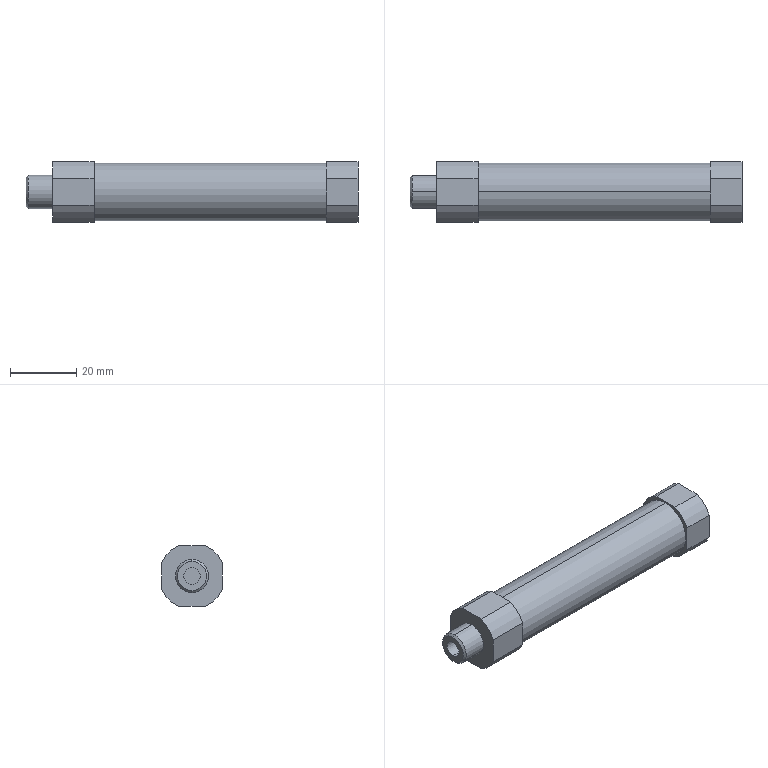Part | SolidWorks | features RefAxis 6, ICE 3, 3DProfileFeature 2, HoleWzd 2, RevCut 1, Revolution 1 | 1 solid | 45 faces | box 100 x 18.3 x 18.3 mm | volume 13157 mm3 | cylinder 20 | plane 15 | cone 10 | commonest cylinder face diameters 20 x8 4.134 x4 5 x2 10 x2 16 x2 17.4 x2
STEP:
#1=CARTESIAN_POINT('',(62.5,0.,-8.));
#2=VERTEX_POINT('',#1);
#3=CARTESIAN_POINT('',(62.5,0.,8.));
#4=VERTEX_POINT('',#3);
#5=CARTESIAN_POINT('',(62.5,0.,0.));
#6=DIRECTION('',(-1.,0.,0.));
#7=DIRECTION('',(0.,0.,1.));
#8=AXIS2_PLACEMENT_3D('',#5,#6,#7);
#9=CIRCLE('',#8,8.);
#10=EDGE_CURVE('',#2,#4,#9,.T.);
#11=ORIENTED_EDGE('',*,*,#10,.F.);
#12=CARTESIAN_POINT('',(12.5,0.,-8.));
#13=VERTEX_POINT('',#12);
#14=CARTESIAN_POINT('',(50.,0.,-8.));
#15=DIRECTION('',(-1.,0.,0.));
#16=VECTOR('',#15,1000.);
#17=LINE('',#14,#16);
#18=EDGE_CURVE('',#2,#13,#17,.T.);
#19=ORIENTED_EDGE('',*,*,#18,.T.);
#20=CARTESIAN_POINT('',(12.5,0.,8.));
#21=VERTEX_POINT('',#20);
#22=CARTESIAN_POINT('',(12.5,0.,0.));
#23=DIRECTION('',(-1.,0.,0.));
#24=DIRECTION('',(0.,0.,1.));
#25=AXIS2_PLACEMENT_3D('',#22,#23,#24);
#26=CIRCLE('',#25,8.);
#27=EDGE_CURVE('',#13,#21,#26,.T.);
#28=ORIENTED_EDGE('',*,*,#27,.T.);
#29=CARTESIAN_POINT('',(50.,0.,8.));
#30=DIRECTION('',(-1.,0.,0.));
#31=VECTOR('',#30,1000.);
#32=LINE('',#29,#31);
#33=EDGE_CURVE('',#4,#21,#32,.T.);
#34=ORIENTED_EDGE('',*,*,#33,.F.);
#35=EDGE_LOOP('',(#11,#19,#28,#34));
#36=FACE_OUTER_BOUND('',#35,.T.);
#37=CARTESIAN_POINT('',(50.,0.,0.));
#38=DIRECTION('',(-1.,0.,0.));
#39=DIRECTION('',(0.,0.,1.));
#40=AXIS2_PLACEMENT_3D('',#37,#38,#39);
#41=CYLINDRICAL_SURFACE('',#40,8.);
#42=ADVANCED_FACE('',(#36),#41,.F.);
#43=CARTESIAN_POINT('',(12.5,0.,-2.5));
#44=VERTEX_POINT('',#43);
#45=CARTESIAN_POINT('',(12.5,0.,2.5));
#46=VERTEX_POINT('',#45);
#47=CARTESIAN_POINT('',(12.5,0.,0.));
#48=DIRECTION('',(-1.,0.,0.));
#49=DIRECTION('',(0.,0.,1.));
#50=AXIS2_PLACEMENT_3D('',#47,#48,#49);
#51=CIRCLE('',#50,2.5);
#52=EDGE_CURVE('',#44,#46,#51,.T.);
#53=ORIENTED_EDGE('',*,*,#52,.F.);
#54=CARTESIAN_POINT('',(-8.,0.,-2.5));
#55=VERTEX_POINT('',#54);
#56=CARTESIAN_POINT('',(50.,0.,-2.5));
#57=DIRECTION('',(-1.,0.,0.));
#58=VECTOR('',#57,1000.);
#59=LINE('',#56,#58);
#60=EDGE_CURVE('',#44,#55,#59,.T.);
#61=ORIENTED_EDGE('',*,*,#60,.T.);
#62=CARTESIAN_POINT('',(-8.,0.,2.5));
#63=VERTEX_POINT('',#62);
#64=CARTESIAN_POINT('',(-8.,0.,0.));
#65=DIRECTION('',(-1.,0.,0.));
#66=DIRECTION('',(0.,0.,1.));
#67=AXIS2_PLACEMENT_3D('',#64,#65,#66);
#68=CIRCLE('',#67,2.5);
#69=EDGE_CURVE('',#55,#63,#68,.T.);
#70=ORIENTED_EDGE('',*,*,#69,.T.);
#71=CARTESIAN_POINT('',(50.,0.,2.5));
#72=DIRECTION('',(-1.,0.,0.));
#73=VECTOR('',#72,1000.);
#74=LINE('',#71,#73);
#75=EDGE_CURVE('',#46,#63,#74,.T.);
#76=ORIENTED_EDGE('',*,*,#75,.F.);
#77=EDGE_LOOP('',(#53,#61,#70,#76));
#78=FACE_OUTER_BOUND('',#77,.T.);
#79=CARTESIAN_POINT('',(50.,0.,0.));
#80=DIRECTION('',(-1.,0.,0.));
#81=DIRECTION('',(0.,0.,1.));
#82=AXIS2_PLACEMENT_3D('',#79,#80,#81);
#83=CYLINDRICAL_SURFACE('',#82,2.5);
#84=ADVANCED_FACE('',(#78),#83,.F.);
#85=CARTESIAN_POINT('',(87.,8.717,-2.067));
#86=VERTEX_POINT('',#85);
#87=CARTESIAN_POINT('',(87.,8.717,2.067));
#88=VERTEX_POINT('',#87);
#89=CARTESIAN_POINT('',(87.,8.717,0.));
#90=DIRECTION('',(0.,1.,0.));
#91=DIRECTION('',(0.,0.,1.));
#92=AXIS2_PLACEMENT_3D('',#89,#90,#91);
#93=CIRCLE('',#92,2.067);
#94=EDGE_CURVE('',#86,#88,#93,.T.);
#95=ORIENTED_EDGE('',*,*,#94,.F.);
#96=CARTESIAN_POINT('',(87.,9.15,-2.5));
#97=VERTEX_POINT('',#96);
#98=CARTESIAN_POINT('',(87.,9.15,-2.5));
#99=DIRECTION('',(0.,0.7071,-0.7071));
#100=VECTOR('',#99,1000.);
#101=LINE('',#98,#100);
#102=EDGE_CURVE('',#86,#97,#101,.T.);
#103=ORIENTED_EDGE('',*,*,#102,.T.);
#104=CARTESIAN_POINT('',(87.,9.15,2.5));
#105=VERTEX_POINT('',#104);
#106=CARTESIAN_POINT('',(87.,9.15,0.));
#107=DIRECTION('',(0.,1.,0.));
#108=DIRECTION('',(0.,0.,1.));
#109=AXIS2_PLACEMENT_3D('',#106,#107,#108);
#110=CIRCLE('',#109,2.5);
#111=EDGE_CURVE('',#97,#105,#110,.T.);
#112=ORIENTED_EDGE('',*,*,#111,.T.);
#113=CARTESIAN_POINT('',(87.,9.15,2.5));
#114=DIRECTION('',(0.,0.7071,0.7071));
#115=VECTOR('',#114,1000.);
#116=LINE('',#113,#115);
#117=EDGE_CURVE('',#88,#105,#116,.T.);
#118=ORIENTED_EDGE('',*,*,#117,.F.);
#119=EDGE_LOOP('',(#95,#103,#112,#118));
#120=FACE_OUTER_BOUND('',#119,.T.);
#121=CARTESIAN_POINT('',(87.,9.15,0.));
#122=DIRECTION('',(0.,1.,0.));
#123=DIRECTION('',(0.,0.,1.));
#124=AXIS2_PLACEMENT_3D('',#121,#122,#123);
#125=CONICAL_SURFACE('',#124,2.5,0.7854);
#126=ADVANCED_FACE('',(#120),#125,.F.);
#127=CARTESIAN_POINT('',(87.,3.65,-2.067));
#128=VERTEX_POINT('',#127);
#129=CARTESIAN_POINT('',(87.,3.65,2.067));
#130=VERTEX_POINT('',#129);
#131=CARTESIAN_POINT('',(87.,3.65,0.));
#132=DIRECTION('',(0.,1.,0.));
#133=DIRECTION('',(0.,0.,1.));
#134=AXIS2_PLACEMENT_3D('',#131,#132,#133);
#135=CIRCLE('',#134,2.067);
#136=EDGE_CURVE('',#128,#130,#135,.T.);
#137=ORIENTED_EDGE('',*,*,#136,.F.);
#138=CARTESIAN_POINT('',(87.,9.15,-2.067));
#139=DIRECTION('',(0.,1.,0.));
#140=VECTOR('',#139,1000.);
#141=LINE('',#138,#140);
#142=EDGE_CURVE('',#128,#86,#141,.T.);
#143=ORIENTED_EDGE('',*,*,#142,.T.);
#144=ORIENTED_EDGE('',*,*,#94,.T.);
#145=CARTESIAN_POINT('',(87.,9.15,2.067));
#146=DIRECTION('',(0.,1.,0.));
#147=VECTOR('',#146,1000.);
#148=LINE('',#145,#147);
#149=EDGE_CURVE('',#130,#88,#148,.T.);
#150=ORIENTED_EDGE('',*,*,#149,.F.);
#151=EDGE_LOOP('',(#137,#143,#144,#150));
#152=FACE_OUTER_BOUND('',#151,.T.);
#153=CARTESIAN_POINT('',(87.,9.15,0.));
#154=DIRECTION('',(0.,1.,0.));
#155=DIRECTION('',(0.,0.,1.));
#156=AXIS2_PLACEMENT_3D('',#153,#154,#155);
#157=CYLINDRICAL_SURFACE('',#156,2.067);
#158=ADVANCED_FACE('',(#152),#157,.F.);
#159=CARTESIAN_POINT('',(87.,2.457,0.));
#160=VERTEX_POINT('',#159);
#161=CARTESIAN_POINT('',(87.,3.65,2.067));
#162=DIRECTION('',(0.,0.5,0.866));
#163=VECTOR('',#162,1000.);
#164=LINE('',#161,#163);
#165=EDGE_CURVE('',#160,#130,#164,.T.);
#166=ORIENTED_EDGE('',*,*,#165,.F.);
#167=CARTESIAN_POINT('',(87.,3.65,-2.067));
#168=DIRECTION('',(0.,0.5,-0.866));
#169=VECTOR('',#168,1000.);
#170=LINE('',#167,#169);
#171=EDGE_CURVE('',#160,#128,#170,.T.);
#172=ORIENTED_EDGE('',*,*,#171,.T.);
#173=ORIENTED_EDGE('',*,*,#136,.T.);
#174=EDGE_LOOP('',(#166,#172,#173));
#175=FACE_OUTER_BOUND('',#174,.T.);
#176=CARTESIAN_POINT('',(87.,3.65,0.));
#177=DIRECTION('',(0.,1.,0.));
#178=DIRECTION('',(0.,0.,1.));
#179=AXIS2_PLACEMENT_3D('',#176,#177,#178);
#180=CONICAL_SURFACE('',#179,2.067,1.047);
#181=ADVANCED_FACE('',(#175),#180,.F.);
#182=CARTESIAN_POINT('',(8.,8.717,-2.067));
#183=VERTEX_POINT('',#182);
#184=CARTESIAN_POINT('',(8.,8.717,2.067));
#185=VERTEX_POINT('',#184);
#186=CARTESIAN_POINT('',(8.,8.717,0.));
#187=DIRECTION('',(0.,1.,0.));
#188=DIRECTION('',(0.,0.,1.));
#189=AXIS2_PLACEMENT_3D('',#186,#187,#188);
#190=CIRCLE('',#189,2.067);
#191=EDGE_CURVE('',#183,#185,#190,.T.);
#192=ORIENTED_EDGE('',*,*,#191,.F.);
#193=CARTESIAN_POINT('',(8.,9.15,-2.5));
#194=VERTEX_POINT('',#193);
#195=CARTESIAN_POINT('',(8.,9.15,-2.5));
#196=DIRECTION('',(0.,0.7071,-0.7071));
#197=VECTOR('',#196,1000.);
#198=LINE('',#195,#197);
#199=EDGE_CURVE('',#183,#194,#198,.T.);
#200=ORIENTED_EDGE('',*,*,#199,.T.);
#201=CARTESIAN_POINT('',(8.,9.15,2.5));
#202=VERTEX_POINT('',#201);
#203=CARTESIAN_POINT('',(8.,9.15,0.));
#204=DIRECTION('',(0.,1.,0.));
#205=DIRECTION('',(0.,0.,1.));
#206=AXIS2_PLACEMENT_3D('',#203,#204,#205);
#207=CIRCLE('',#206,2.5);
#208=EDGE_CURVE('',#194,#202,#207,.T.);
#209=ORIENTED_EDGE('',*,*,#208,.T.);
#210=CARTESIAN_POINT('',(8.,9.15,2.5));
#211=DIRECTION('',(0.,0.7071,0.7071));
#212=VECTOR('',#211,1000.);
#213=LINE('',#210,#212);
#214=EDGE_CURVE('',#185,#202,#213,.T.);
#215=ORIENTED_EDGE('',*,*,#214,.F.);
#216=EDGE_LOOP('',(#192,#200,#209,#215));
#217=FACE_OUTER_BOUND('',#216,.T.);
#218=CARTESIAN_POINT('',(8.,9.15,0.));
#219=DIRECTION('',(0.,1.,0.));
#220=DIRECTION('',(0.,0.,1.));
#221=AXIS2_PLACEMENT_3D('',#218,#219,#220);
#222=CONICAL_SURFACE('',#221,2.5,0.7854);
#223=ADVANCED_FACE('',(#217),#222,.F.);
#224=CARTESIAN_POINT('',(8.,3.65,-2.067));
#225=VERTEX_POINT('',#224);
#226=CARTESIAN_POINT('',(8.,3.65,2.067));
#227=VERTEX_POINT('',#226);
#228=CARTESIAN_POINT('',(8.,3.65,0.));
#229=DIRECTION('',(0.,1.,0.));
#230=DIRECTION('',(0.,0.,1.));
#231=AXIS2_PLACEMENT_3D('',#228,#229,#230);
#232=CIRCLE('',#231,2.067);
#233=EDGE_CURVE('',#225,#227,#232,.T.);
#234=ORIENTED_EDGE('',*,*,#233,.F.);
#235=CARTESIAN_POINT('',(8.,9.15,-2.067));
#236=DIRECTION('',(0.,1.,0.));
#237=VECTOR('',#236,1000.);
#238=LINE('',#235,#237);
#239=EDGE_CURVE('',#225,#183,#238,.T.);
#240=ORIENTED_EDGE('',*,*,#239,.T.);
#241=ORIENTED_EDGE('',*,*,#191,.T.);
#242=CARTESIAN_POINT('',(8.,9.15,2.067));
#243=DIRECTION('',(0.,1.,0.));
#244=VECTOR('',#243,1000.);
#245=LINE('',#242,#244);
#246=EDGE_CURVE('',#227,#185,#245,.T.);
#247=ORIENTED_EDGE('',*,*,#246,.F.);
#248=EDGE_LOOP('',(#234,#240,#241,#247));
#249=FACE_OUTER_BOUND('',#248,.T.);
#250=CARTESIAN_POINT('',(8.,9.15,0.));
#251=DIRECTION('',(0.,1.,0.));
#252=DIRECTION('',(0.,0.,1.));
#253=AXIS2_PLACEMENT_3D('',#250,#251,#252);
#254=CYLINDRICAL_SURFACE('',#253,2.067);
#255=ADVANCED_FACE('',(#249),#254,.F.);
#256=CARTESIAN_POINT('',(82.5,0.,-8.7));
#257=VERTEX_POINT('',#256);
#258=CARTESIAN_POINT('',(82.5,0.,8.7));
#259=VERTEX_POINT('',#258);
#260=CARTESIAN_POINT('',(82.5,0.,0.));
#261=DIRECTION('',(1.,0.,0.));
#262=DIRECTION('',(0.,0.,-1.));
#263=AXIS2_PLACEMENT_3D('',#260,#261,#262);
#264=CIRCLE('',#263,8.7);
#265=EDGE_CURVE('',#257,#259,#264,.T.);
#266=ORIENTED_EDGE('',*,*,#265,.F.);
#267=CARTESIAN_POINT('',(12.5,0.,-8.7));
#268=VERTEX_POINT('',#267);
#269=CARTESIAN_POINT('',(82.5,0.,-8.7));
#270=DIRECTION('',(-1.,0.,0.));
#271=VECTOR('',#270,1000.);
#272=LINE('',#269,#271);
#273=EDGE_CURVE('',#257,#268,#272,.T.);
#274=ORIENTED_EDGE('',*,*,#273,.T.);
#275=CARTESIAN_POINT('',(12.5,0.,8.7));
#276=VERTEX_POINT('',#275);
#277=CARTESIAN_POINT('',(12.5,0.,0.));
#278=DIRECTION('',(1.,0.,0.));
#279=DIRECTION('',(0.,0.,-1.));
#280=AXIS2_PLACEMENT_3D('',#277,#278,#279);
#281=CIRCLE('',#280,8.7);
#282=EDGE_CURVE('',#268,#276,#281,.T.);
#283=ORIENTED_EDGE('',*,*,#282,.T.);
#284=CARTESIAN_POINT('',(82.5,0.,8.7));
#285=DIRECTION('',(-1.,0.,0.));
#286=VECTOR('',#285,1000.);
#287=LINE('',#284,#286);
#288=EDGE_CURVE('',#259,#276,#287,.T.);
#289=ORIENTED_EDGE('',*,*,#288,.F.);
#290=EDGE_LOOP('',(#266,#274,#283,#289));
#291=FACE_OUTER_BOUND('',#290,.T.);
#292=CARTESIAN_POINT('',(82.5,0.,0.));
#293=DIRECTION('',(-1.,0.,0.));
#294=DIRECTION('',(0.,0.,1.));
#295=AXIS2_PLACEMENT_3D('',#292,#293,#294);
#296=CYLINDRICAL_SURFACE('',#295,8.7);
#297=ADVANCED_FACE('',(#291),#296,.T.);
#298=CARTESIAN_POINT('',(0.,0.,-5.));
#299=VERTEX_POINT('',#298);
#300=CARTESIAN_POINT('',(0.,0.,5.));
#301=VERTEX_POINT('',#300);
#302=CARTESIAN_POINT('',(0.,0.,0.));
#303=DIRECTION('',(1.,0.,0.));
#304=DIRECTION('',(0.,0.,-1.));
#305=AXIS2_PLACEMENT_3D('',#302,#303,#304);
#306=CIRCLE('',#305,5.);
#307=EDGE_CURVE('',#299,#301,#306,.T.);
#308=ORIENTED_EDGE('',*,*,#307,.F.);
#309=CARTESIAN_POINT('',(-7.386,0.,-5.));
#310=VERTEX_POINT('',#309);
#311=CARTESIAN_POINT('',(0.,0.,-5.));
#312=DIRECTION('',(-1.,0.,0.));
#313=VECTOR('',#312,1000.);
#314=LINE('',#311,#313);
#315=EDGE_CURVE('',#299,#310,#314,.T.);
#316=ORIENTED_EDGE('',*,*,#315,.T.);
#317=CARTESIAN_POINT('',(-7.386,0.,5.));
#318=VERTEX_POINT('',#317);
#319=CARTESIAN_POINT('',(-7.386,0.,0.));
#320=DIRECTION('',(-1.,0.,0.));
#321=DIRECTION('',(0.,0.,1.));
#322=AXIS2_PLACEMENT_3D('',#319,#320,#321);
#323=CIRCLE('',#322,5.);
#324=EDGE_CURVE('',#318,#310,#323,.T.);
#325=ORIENTED_EDGE('',*,*,#324,.F.);
#326=CARTESIAN_POINT('',(0.,0.,5.));
#327=DIRECTION('',(-1.,0.,0.));
#328=VECTOR('',#327,1000.);
#329=LINE('',#326,#328);
#330=EDGE_CURVE('',#301,#318,#329,.T.);
#331=ORIENTED_EDGE('',*,*,#330,.F.);
#332=EDGE_LOOP('',(#308,#316,#325,#331));
#333=FACE_OUTER_BOUND('',#332,.T.);
#334=CARTESIAN_POINT('',(0.,0.,0.));
#335=DIRECTION('',(-1.,0.,0.));
#336=DIRECTION('',(0.,0.,1.));
#337=AXIS2_PLACEMENT_3D('',#334,#335,#336);
#338=CYLINDRICAL_SURFACE('',#337,5.);
#339=ADVANCED_FACE('',(#333),#338,.T.);
#340=CARTESIAN_POINT('',(-8.,0.,4.386));
#341=VERTEX_POINT('',#340);
#342=CARTESIAN_POINT('',(-8.,0.,-4.386));
#343=VERTEX_POINT('',#342);
#344=CARTESIAN_POINT('',(-8.,0.,0.));
#345=DIRECTION('',(-1.,0.,0.));
#346=DIRECTION('',(0.,0.,1.));
#347=AXIS2_PLACEMENT_3D('',#344,#345,#346);
#348=CIRCLE('',#347,4.386);
#349=EDGE_CURVE('',#341,#343,#348,.T.);
#350=ORIENTED_EDGE('',*,*,#349,.F.);
#351=CARTESIAN_POINT('',(-7.386,0.,5.));
#352=DIRECTION('',(0.7071,0.,0.7071));
#353=VECTOR('',#352,1000.);
#354=LINE('',#351,#353);
#355=EDGE_CURVE('',#341,#318,#354,.T.);
#356=ORIENTED_EDGE('',*,*,#355,.T.);
#357=ORIENTED_EDGE('',*,*,#324,.T.);
#358=CARTESIAN_POINT('',(-7.386,0.,-5.));
#359=DIRECTION('',(0.7071,0.,-0.7071));
#360=VECTOR('',#359,1000.);
#361=LINE('',#358,#360);
#362=EDGE_CURVE('',#343,#310,#361,.T.);
#363=ORIENTED_EDGE('',*,*,#362,.F.);
#364=EDGE_LOOP('',(#350,#356,#357,#363));
#365=FACE_OUTER_BOUND('',#364,.T.);
#366=CARTESIAN_POINT('',(-7.386,0.,0.));
#367=DIRECTION('',(1.,0.,0.));
#368=DIRECTION('',(0.,0.,-1.));
#369=AXIS2_PLACEMENT_3D('',#366,#367,#368);
#370=CONICAL_SURFACE('',#369,5.,0.7854);
#371=ADVANCED_FACE('',(#365),#370,.T.);
#372=CARTESIAN_POINT('',(8.,2.499,-0.07328));
#373=VERTEX_POINT('',#372);
#374=CARTESIAN_POINT('',(8.,2.499,0.07328));
#375=VERTEX_POINT('',#374);
#376=CARTESIAN_POINT('',(8.,2.499,-0.07328));
#377=CARTESIAN_POINT('',(7.998,2.499,-0.07328));
#378=CARTESIAN_POINT('',(7.995,2.499,-0.07316));
#379=CARTESIAN_POINT('',(7.993,2.499,-0.07293));
#380=CARTESIAN_POINT('',(7.987,2.499,-0.0724));
#381=CARTESIAN_POINT('',(7.982,2.499,-0.07129));
#382=CARTESIAN_POINT('',(7.977,2.499,-0.06961));
#383=CARTESIAN_POINT('',(7.968,2.499,-0.06701));
#384=CARTESIAN_POINT('',(7.961,2.499,-0.06299));
#385=CARTESIAN_POINT('',(7.954,2.499,-0.05786));
#386=CARTESIAN_POINT('',(7.947,2.499,-0.05273));
#387=CARTESIAN_POINT('',(7.941,2.5,-0.04635));
#388=CARTESIAN_POINT('',(7.937,2.5,-0.03923));
#389=CARTESIAN_POINT('',(7.932,2.5,-0.03228));
#390=CARTESIAN_POINT('',(7.929,2.5,-0.02443));
#391=CARTESIAN_POINT('',(7.927,2.5,-0.01636));
#392=CARTESIAN_POINT('',(7.925,2.5,-0.008479));
#393=CARTESIAN_POINT('',(7.924,2.5,-0.0001614));
#394=CARTESIAN_POINT('',(7.925,2.5,0.007886));
#395=CARTESIAN_POINT('',(7.926,2.5,0.01584));
#396=CARTESIAN_POINT('',(7.928,2.5,0.02374));
#397=CARTESIAN_POINT('',(7.932,2.5,0.03096));
#398=CARTESIAN_POINT('',(7.935,2.5,0.03821));
#399=CARTESIAN_POINT('',(7.94,2.5,0.04496));
#400=CARTESIAN_POINT('',(7.946,2.499,0.0507));
#401=CARTESIAN_POINT('',(7.951,2.499,0.05654));
#402=CARTESIAN_POINT('',(7.958,2.499,0.06149));
#403=CARTESIAN_POINT('',(7.966,2.499,0.06516));
#404=CARTESIAN_POINT('',(7.973,2.499,0.06893));
#405=CARTESIAN_POINT('',(7.981,2.499,0.07146));
#406=CARTESIAN_POINT('',(7.99,2.499,0.07259));
#407=CARTESIAN_POINT('',(7.993,2.499,0.07305));
#408=CARTESIAN_POINT('',(7.997,2.499,0.07328));
#409=CARTESIAN_POINT('',(8.,2.499,0.07328));
#410=B_SPLINE_CURVE_WITH_KNOTS('',3,(#376,#377,#378,#379,#380,#381,#382,#383,#384,#385,#386,#387,#388,#389,#390,#391,#392,#393,#394,#395,#396,#397,#398,#399,#400,#401,#402,#403,#404,#405,#406,#407,#408,#409),.UNSPECIFIED.,.F.,.F.,(4,3,3,3,3,3,3,3,3,3,3,4),(0.0004402,0.0004476,0.0004639,0.0004894,0.0005148,0.0005397,0.000564,0.000588,0.0006121,0.0006366,0.0006618,0.0006721),.UNSPECIFIED.);
#411=EDGE_CURVE('',#373,#375,#410,.T.);
#412=ORIENTED_EDGE('',*,*,#411,.F.);
#413=CARTESIAN_POINT('',(8.,3.65,-2.067));
#414=DIRECTION('',(0.,0.5,-0.866));
#415=VECTOR('',#414,1000.);
#416=LINE('',#413,#415);
#417=EDGE_CURVE('',#373,#225,#416,.T.);
#418=ORIENTED_EDGE('',*,*,#417,.T.);
#419=ORIENTED_EDGE('',*,*,#233,.T.);
#420=CARTESIAN_POINT('',(8.,3.65,2.067));
#421=DIRECTION('',(0.,0.5,0.866));
#422=VECTOR('',#421,1000.);
#423=LINE('',#420,#422);
#424=EDGE_CURVE('',#375,#227,#423,.T.);
#425=ORIENTED_EDGE('',*,*,#424,.F.);
#426=EDGE_LOOP('',(#412,#418,#419,#425));
#427=FACE_OUTER_BOUND('',#426,.T.);
#428=CARTESIAN_POINT('',(8.,3.65,0.));
#429=DIRECTION('',(0.,1.,0.));
#430=DIRECTION('',(0.,0.,1.));
#431=AXIS2_PLACEMENT_3D('',#428,#429,#430);
#432=CONICAL_SURFACE('',#431,2.067,1.047);
#433=ADVANCED_FACE('',(#427),#432,.F.);
#434=CARTESIAN_POINT('',(-8.,0.,0.));
#435=DIRECTION('',(-1.,0.,0.));
#436=DIRECTION('',(0.,0.,1.));
#437=AXIS2_PLACEMENT_3D('',#434,#435,#436);
#438=CIRCLE('',#437,4.386);
#439=EDGE_CURVE('',#343,#341,#438,.T.);
#440=ORIENTED_EDGE('',*,*,#439,.T.);
#441=ORIENTED_EDGE('',*,*,#349,.T.);
#442=EDGE_LOOP('',(#440,#441));
#443=FACE_OUTER_BOUND('',#442,.T.);
#444=CARTESIAN_POINT('',(-8.,0.,0.));
#445=DIRECTION('',(-1.,0.,0.));
#446=DIRECTION('',(0.,0.,1.));
#447=AXIS2_PLACEMENT_3D('',#444,#445,#446);
#448=CIRCLE('',#447,2.5);
#449=EDGE_CURVE('',#63,#55,#448,.T.);
#450=ORIENTED_EDGE('',*,*,#449,.F.);
#451=ORIENTED_EDGE('',*,*,#69,.F.);
#452=EDGE_LOOP('',(#450,#451));
#453=FACE_BOUND('',#452,.T.);
#454=CARTESIAN_POINT('',(-8.,0.,0.));
#455=DIRECTION('',(1.,0.,0.));
#456=DIRECTION('',(0.,0.,-1.));
#457=AXIS2_PLACEMENT_3D('',#454,#455,#456);
#458=PLANE('',#457);
#459=ADVANCED_FACE('',(#443,#453),#458,.F.);
#460=ORIENTED_EDGE('',*,*,#417,.F.);
#461=CARTESIAN_POINT('',(8.,2.499,0.07328));
#462=CARTESIAN_POINT('',(8.005,2.499,0.07328));
#463=CARTESIAN_POINT('',(8.01,2.499,0.07276));
#464=CARTESIAN_POINT('',(8.015,2.499,0.07173));
#465=CARTESIAN_POINT('',(8.024,2.499,0.07002));
#466=CARTESIAN_POINT('',(8.032,2.499,0.06682));
#467=CARTESIAN_POINT('',(8.039,2.499,0.06238));
#468=CARTESIAN_POINT('',(8.047,2.499,0.05798));
#469=CARTESIAN_POINT('',(8.053,2.499,0.05224));
#470=CARTESIAN_POINT('',(8.059,2.5,0.04563));
#471=CARTESIAN_POINT('',(8.064,2.5,0.03915));
#472=CARTESIAN_POINT('',(8.068,2.5,0.03166));
#473=CARTESIAN_POINT('',(8.071,2.5,0.02377));
#474=CARTESIAN_POINT('',(8.074,2.5,0.01608));
#475=CARTESIAN_POINT('',(8.075,2.5,0.00781));
#476=CARTESIAN_POINT('',(8.075,2.5,-0.0003406));
#477=CARTESIAN_POINT('',(8.075,2.5,-0.008355));
#478=CARTESIAN_POINT('',(8.074,2.5,-0.01647));
#479=CARTESIAN_POINT('',(8.071,2.5,-0.02402));
#480=CARTESIAN_POINT('',(8.068,2.5,-0.03157));
#481=CARTESIAN_POINT('',(8.064,2.5,-0.03876));
#482=CARTESIAN_POINT('',(8.059,2.5,-0.04502));
#483=CARTESIAN_POINT('',(8.054,2.499,-0.05138));
#484=CARTESIAN_POINT('',(8.048,2.499,-0.05695));
#485=CARTESIAN_POINT('',(8.041,2.499,-0.06133));
#486=CARTESIAN_POINT('',(8.034,2.499,-0.06581));
#487=CARTESIAN_POINT('',(8.026,2.499,-0.06916));
#488=CARTESIAN_POINT('',(8.018,2.499,-0.07112));
#489=CARTESIAN_POINT('',(8.012,2.499,-0.07255));
#490=CARTESIAN_POINT('',(8.006,2.499,-0.07328));
#491=CARTESIAN_POINT('',(8.,2.499,-0.07328));
#492=B_SPLINE_CURVE_WITH_KNOTS('',3,(#461,#462,#463,#464,#465,#466,#467,#468,#469,#470,#471,#472,#473,#474,#475,#476,#477,#478,#479,#480,#481,#482,#483,#484,#485,#486,#487,#488,#489,#490,#491),.UNSPECIFIED.,.F.,.F.,(4,3,3,3,3,3,3,3,3,3,4),(0.0002082,0.0002236,0.0002495,0.0002751,0.0003002,0.0003246,0.0003486,0.0003726,0.000397,0.000422,0.0004402),.UNSPECIFIED.);
#493=EDGE_CURVE('',#375,#373,#492,.T.);
#494=ORIENTED_EDGE('',*,*,#493,.F.);
#495=ORIENTED_EDGE('',*,*,#424,.T.);
#496=CARTESIAN_POINT('',(8.,3.65,0.));
#497=DIRECTION('',(0.,1.,0.));
#498=DIRECTION('',(0.,0.,1.));
#499=AXIS2_PLACEMENT_3D('',#496,#497,#498);
#500=CIRCLE('',#499,2.067);
#501=EDGE_CURVE('',#227,#225,#500,.T.);
#502=ORIENTED_EDGE('',*,*,#501,.T.);
#503=EDGE_LOOP('',(#460,#494,#495,#502));
#504=FACE_OUTER_BOUND('',#503,.T.);
#505=CARTESIAN_POINT('',(8.,3.65,0.));
#506=DIRECTION('',(0.,1.,0.));
#507=DIRECTION('',(0.,0.,1.));
#508=AXIS2_PLACEMENT_3D('',#505,#506,#507);
#509=CONICAL_SURFACE('',#508,2.067,1.047);
#510=ADVANCED_FACE('',(#504),#509,.F.);
#511=CARTESIAN_POINT('',(12.5,-4.035,9.15));
#512=VERTEX_POINT('',#511);
#513=CARTESIAN_POINT('',(12.5,-9.15,4.035));
#514=VERTEX_POINT('',#513);
#515=CARTESIAN_POINT('',(12.5,0.,0.));
#516=DIRECTION('',(1.,0.,0.));
#517=DIRECTION('',(0.,0.,-1.));
#518=AXIS2_PLACEMENT_3D('',#515,#516,#517);
#519=CIRCLE('',#518,10.);
#520=EDGE_CURVE('',#512,#514,#519,.T.);
#521=ORIENTED_EDGE('',*,*,#520,.T.);
#522=CARTESIAN_POINT('',(12.5,-9.15,-4.035));
#523=VERTEX_POINT('',#522);
#524=CARTESIAN_POINT('',(12.5,-9.15,4.035));
#525=DIRECTION('',(0.,0.,-1.));
#526=VECTOR('',#525,1000.);
#527=LINE('',#524,#526);
#528=EDGE_CURVE('',#514,#523,#527,.T.);
#529=ORIENTED_EDGE('',*,*,#528,.T.);
#530=CARTESIAN_POINT('',(12.5,-4.035,-9.15));
#531=VERTEX_POINT('',#530);
#532=CARTESIAN_POINT('',(12.5,0.,0.));
#533=DIRECTION('',(1.,0.,0.));
#534=DIRECTION('',(0.,0.,-1.));
#535=AXIS2_PLACEMENT_3D('',#532,#533,#534);
#536=CIRCLE('',#535,10.);
#537=EDGE_CURVE('',#523,#531,#536,.T.);
#538=ORIENTED_EDGE('',*,*,#537,.T.);
#539=CARTESIAN_POINT('',(12.5,4.035,-9.15));
#540=VERTEX_POINT('',#539);
#541=CARTESIAN_POINT('',(12.5,-4.035,-9.15));
#542=DIRECTION('',(0.,1.,0.));
#543=VECTOR('',#542,1000.);
#544=LINE('',#541,#543);
#545=EDGE_CURVE('',#531,#540,#544,.T.);
#546=ORIENTED_EDGE('',*,*,#545,.T.);
#547=CARTESIAN_POINT('',(12.5,9.15,-4.035));
#548=VERTEX_POINT('',#547);
#549=CARTESIAN_POINT('',(12.5,0.,0.));
#550=DIRECTION('',(1.,0.,0.));
#551=DIRECTION('',(0.,0.,-1.));
#552=AXIS2_PLACEMENT_3D('',#549,#550,#551);
#553=CIRCLE('',#552,10.);
#554=EDGE_CURVE('',#540,#548,#553,.T.);
#555=ORIENTED_EDGE('',*,*,#554,.T.);
#556=CARTESIAN_POINT('',(12.5,9.15,4.035));
#557=VERTEX_POINT('',#556);
#558=CARTESIAN_POINT('',(12.5,9.15,-4.035));
#559=DIRECTION('',(0.,0.,1.));
#560=VECTOR('',#559,1000.);
#561=LINE('',#558,#560);
#562=EDGE_CURVE('',#548,#557,#561,.T.);
#563=ORIENTED_EDGE('',*,*,#562,.T.);
#564=CARTESIAN_POINT('',(12.5,4.035,9.15));
#565=VERTEX_POINT('',#564);
#566=CARTESIAN_POINT('',(12.5,0.,0.));
#567=DIRECTION('',(1.,0.,0.));
#568=DIRECTION('',(0.,0.,-1.));
#569=AXIS2_PLACEMENT_3D('',#566,#567,#568);
#570=CIRCLE('',#569,10.);
#571=EDGE_CURVE('',#557,#565,#570,.T.);
#572=ORIENTED_EDGE('',*,*,#571,.T.);
#573=CARTESIAN_POINT('',(12.5,4.035,9.15));
#574=DIRECTION('',(0.,-1.,0.));
#575=VECTOR('',#574,1000.);
#576=LINE('',#573,#575);
#577=EDGE_CURVE('',#565,#512,#576,.T.);
#578=ORIENTED_EDGE('',*,*,#577,.T.);
#579=EDGE_LOOP('',(#521,#529,#538,#546,#555,#563,#572,#578));
#580=FACE_OUTER_BOUND('',#579,.T.);
#581=CARTESIAN_POINT('',(12.5,0.,0.));
#582=DIRECTION('',(1.,0.,0.));
#583=DIRECTION('',(0.,0.,-1.));
#584=AXIS2_PLACEMENT_3D('',#581,#582,#583);
#585=CIRCLE('',#584,8.7);
#586=EDGE_CURVE('',#276,#268,#585,.T.);
#587=ORIENTED_EDGE('',*,*,#586,.F.);
#588=ORIENTED_EDGE('',*,*,#282,.F.);
#589=EDGE_LOOP('',(#587,#588));
#590=FACE_BOUND('',#589,.T.);
#591=CARTESIAN_POINT('',(12.5,0.,0.));
#592=DIRECTION('',(1.,0.,0.));
#593=DIRECTION('',(0.,0.,-1.));
#594=AXIS2_PLACEMENT_3D('',#591,#592,#593);
#595=PLANE('',#594);
#596=ADVANCED_FACE('',(#580,#590),#595,.T.);
#597=ORIENTED_EDGE('',*,*,#355,.F.);
#598=ORIENTED_EDGE('',*,*,#439,.F.);
#599=ORIENTED_EDGE('',*,*,#362,.T.);
#600=CARTESIAN_POINT('',(-7.386,0.,0.));
#601=DIRECTION('',(-1.,0.,0.));
#602=DIRECTION('',(0.,0.,1.));
#603=AXIS2_PLACEMENT_3D('',#600,#601,#602);
#604=CIRCLE('',#603,5.);
#605=EDGE_CURVE('',#310,#318,#604,.T.);
#606=ORIENTED_EDGE('',*,*,#605,.T.);
#607=EDGE_LOOP('',(#597,#598,#599,#606));
#608=FACE_OUTER_BOUND('',#607,.T.);
#609=CARTESIAN_POINT('',(-7.386,0.,0.));
#610=DIRECTION('',(1.,0.,0.));
#611=DIRECTION('',(0.,0.,-1.));
#612=AXIS2_PLACEMENT_3D('',#609,#610,#611);
#613=CONICAL_SURFACE('',#612,5.,0.7854);
#614=ADVANCED_FACE('',(#608),#613,.T.);
#615=ORIENTED_EDGE('',*,*,#315,.F.);
#616=CARTESIAN_POINT('',(0.,0.,0.));
#617=DIRECTION('',(1.,0.,0.));
#618=DIRECTION('',(0.,0.,-1.));
#619=AXIS2_PLACEMENT_3D('',#616,#617,#618);
#620=CIRCLE('',#619,5.);
#621=EDGE_CURVE('',#301,#299,#620,.T.);
#622=ORIENTED_EDGE('',*,*,#621,.F.);
#623=ORIENTED_EDGE('',*,*,#330,.T.);
#624=ORIENTED_EDGE('',*,*,#605,.F.);
#625=EDGE_LOOP('',(#615,#622,#623,#624));
#626=FACE_OUTER_BOUND('',#625,.T.);
#627=CARTESIAN_POINT('',(0.,0.,0.));
#628=DIRECTION('',(-1.,0.,0.));
#629=DIRECTION('',(0.,0.,1.));
#630=AXIS2_PLACEMENT_3D('',#627,#628,#629);
#631=CYLINDRICAL_SURFACE('',#630,5.);
#632=ADVANCED_FACE('',(#626),#631,.T.);
#633=CARTESIAN_POINT('',(0.,-4.035,9.15));
#634=VERTEX_POINT('',#633);
#635=CARTESIAN_POINT('',(0.,-9.15,4.035));
#636=VERTEX_POINT('',#635);
#637=CARTESIAN_POINT('',(0.,0.,0.));
#638=DIRECTION('',(1.,0.,0.));
#639=DIRECTION('',(0.,0.,-1.));
#640=AXIS2_PLACEMENT_3D('',#637,#638,#639);
#641=CIRCLE('',#640,10.);
#642=EDGE_CURVE('',#634,#636,#641,.T.);
#643=ORIENTED_EDGE('',*,*,#642,.F.);
#644=CARTESIAN_POINT('',(0.,4.035,9.15));
#645=VERTEX_POINT('',#644);
#646=CARTESIAN_POINT('',(0.,4.035,9.15));
#647=DIRECTION('',(0.,-1.,0.));
#648=VECTOR('',#647,1000.);
#649=LINE('',#646,#648);
#650=EDGE_CURVE('',#645,#634,#649,.T.);
#651=ORIENTED_EDGE('',*,*,#650,.F.);
#652=CARTESIAN_POINT('',(0.,9.15,4.035));
#653=VERTEX_POINT('',#652);
#654=CARTESIAN_POINT('',(0.,0.,0.));
#655=DIRECTION('',(1.,0.,0.));
#656=DIRECTION('',(0.,0.,-1.));
#657=AXIS2_PLACEMENT_3D('',#654,#655,#656);
#658=CIRCLE('',#657,10.);
#659=EDGE_CURVE('',#653,#645,#658,.T.);
#660=ORIENTED_EDGE('',*,*,#659,.F.);
#661=CARTESIAN_POINT('',(0.,9.15,-4.035));
#662=VERTEX_POINT('',#661);
#663=CARTESIAN_POINT('',(0.,9.15,-4.035));
#664=DIRECTION('',(0.,0.,1.));
#665=VECTOR('',#664,1000.);
#666=LINE('',#663,#665);
#667=EDGE_CURVE('',#662,#653,#666,.T.);
#668=ORIENTED_EDGE('',*,*,#667,.F.);
#669=CARTESIAN_POINT('',(0.,4.035,-9.15));
#670=VERTEX_POINT('',#669);
#671=CARTESIAN_POINT('',(0.,0.,0.));
#672=DIRECTION('',(1.,0.,0.));
#673=DIRECTION('',(0.,0.,-1.));
#674=AXIS2_PLACEMENT_3D('',#671,#672,#673);
#675=CIRCLE('',#674,10.);
#676=EDGE_CURVE('',#670,#662,#675,.T.);
#677=ORIENTED_EDGE('',*,*,#676,.F.);
#678=CARTESIAN_POINT('',(0.,-4.035,-9.15));
#679=VERTEX_POINT('',#678);
#680=CARTESIAN_POINT('',(0.,-4.035,-9.15));
#681=DIRECTION('',(0.,1.,0.));
#682=VECTOR('',#681,1000.);
#683=LINE('',#680,#682);
#684=EDGE_CURVE('',#679,#670,#683,.T.);
#685=ORIENTED_EDGE('',*,*,#684,.F.);
#686=CARTESIAN_POINT('',(0.,-9.15,-4.035));
#687=VERTEX_POINT('',#686);
#688=CARTESIAN_POINT('',(0.,0.,0.));
#689=DIRECTION('',(1.,0.,0.));
#690=DIRECTION('',(0.,0.,-1.));
#691=AXIS2_PLACEMENT_3D('',#688,#689,#690);
#692=CIRCLE('',#691,10.);
#693=EDGE_CURVE('',#687,#679,#692,.T.);
#694=ORIENTED_EDGE('',*,*,#693,.F.);
#695=CARTESIAN_POINT('',(0.,-9.15,4.035));
#696=DIRECTION('',(0.,0.,-1.));
#697=VECTOR('',#696,1000.);
#698=LINE('',#695,#697);
#699=EDGE_CURVE('',#636,#687,#698,.T.);
#700=ORIENTED_EDGE('',*,*,#699,.F.);
#701=EDGE_LOOP('',(#643,#651,#660,#668,#677,#685,#694,#700));
#702=FACE_OUTER_BOUND('',#701,.T.);
#703=ORIENTED_EDGE('',*,*,#621,.T.);
#704=ORIENTED_EDGE('',*,*,#307,.T.);
#705=EDGE_LOOP('',(#703,#704));
#706=FACE_BOUND('',#705,.T.);
#707=CARTESIAN_POINT('',(0.,0.,0.));
#708=DIRECTION('',(1.,0.,0.));
#709=DIRECTION('',(0.,0.,-1.));
#710=AXIS2_PLACEMENT_3D('',#707,#708,#709);
#711=PLANE('',#710);
#712=ADVANCED_FACE('',(#702,#706),#711,.F.);
#713=ORIENTED_EDGE('',*,*,#642,.T.);
#714=CARTESIAN_POINT('',(12.5,-9.15,4.035));
#715=DIRECTION('',(-1.,0.,0.));
#716=VECTOR('',#715,1000.);
#717=LINE('',#714,#716);
#718=EDGE_CURVE('',#514,#636,#717,.T.);
#719=ORIENTED_EDGE('',*,*,#718,.F.);
#720=ORIENTED_EDGE('',*,*,#520,.F.);
#721=CARTESIAN_POINT('',(12.5,-4.035,9.15));
#722=DIRECTION('',(-1.,0.,0.));
#723=VECTOR('',#722,1000.);
#724=LINE('',#721,#723);
#725=EDGE_CURVE('',#512,#634,#724,.T.);
#726=ORIENTED_EDGE('',*,*,#725,.T.);
#727=EDGE_LOOP('',(#713,#719,#720,#726));
#728=FACE_OUTER_BOUND('',#727,.T.);
#729=CARTESIAN_POINT('',(12.5,0.,0.));
#730=DIRECTION('',(-1.,0.,0.));
#731=DIRECTION('',(0.,0.,1.));
#732=AXIS2_PLACEMENT_3D('',#729,#730,#731);
#733=CYLINDRICAL_SURFACE('',#732,10.);
#734=ADVANCED_FACE('',(#728),#733,.T.);
#735=ORIENTED_EDGE('',*,*,#699,.T.);
#736=CARTESIAN_POINT('',(12.5,-9.15,-4.035));
#737=DIRECTION('',(-1.,0.,0.));
#738=VECTOR('',#737,1000.);
#739=LINE('',#736,#738);
#740=EDGE_CURVE('',#523,#687,#739,.T.);
#741=ORIENTED_EDGE('',*,*,#740,.F.);
#742=ORIENTED_EDGE('',*,*,#528,.F.);
#743=ORIENTED_EDGE('',*,*,#718,.T.);
#744=EDGE_LOOP('',(#735,#741,#742,#743));
#745=FACE_OUTER_BOUND('',#744,.T.);
#746=CARTESIAN_POINT('',(12.5,-9.15,4.035));
#747=DIRECTION('',(0.,1.,0.));
#748=DIRECTION('',(0.,0.,1.));
#749=AXIS2_PLACEMENT_3D('',#746,#747,#748);
#750=PLANE('',#749);
#751=ADVANCED_FACE('',(#745),#750,.F.);
#752=ORIENTED_EDGE('',*,*,#693,.T.);
#753=CARTESIAN_POINT('',(12.5,-4.035,-9.15));
#754=DIRECTION('',(-1.,0.,0.));
#755=VECTOR('',#754,1000.);
#756=LINE('',#753,#755);
#757=EDGE_CURVE('',#531,#679,#756,.T.);
#758=ORIENTED_EDGE('',*,*,#757,.F.);
#759=ORIENTED_EDGE('',*,*,#537,.F.);
#760=ORIENTED_EDGE('',*,*,#740,.T.);
#761=EDGE_LOOP('',(#752,#758,#759,#760));
#762=FACE_OUTER_BOUND('',#761,.T.);
#763=CARTESIAN_POINT('',(12.5,0.,0.));
#764=DIRECTION('',(-1.,0.,0.));
#765=DIRECTION('',(0.,0.,1.));
#766=AXIS2_PLACEMENT_3D('',#763,#764,#765);
#767=CYLINDRICAL_SURFACE('',#766,10.);
#768=ADVANCED_FACE('',(#762),#767,.T.);
#769=ORIENTED_EDGE('',*,*,#684,.T.);
#770=CARTESIAN_POINT('',(12.5,4.035,-9.15));
#771=DIRECTION('',(-1.,0.,0.));
#772=VECTOR('',#771,1000.);
#773=LINE('',#770,#772);
#774=EDGE_CURVE('',#540,#670,#773,.T.);
#775=ORIENTED_EDGE('',*,*,#774,.F.);
#776=ORIENTED_EDGE('',*,*,#545,.F.);
#777=ORIENTED_EDGE('',*,*,#757,.T.);
#778=EDGE_LOOP('',(#769,#775,#776,#777));
#779=FACE_OUTER_BOUND('',#778,.T.);
#780=CARTESIAN_POINT('',(12.5,-4.035,-9.15));
#781=DIRECTION('',(0.,0.,1.));
#782=DIRECTION('',(1.,0.,0.));
#783=AXIS2_PLACEMENT_3D('',#780,#781,#782);
#784=PLANE('',#783);
#785=ADVANCED_FACE('',(#779),#784,.F.);
#786=ORIENTED_EDGE('',*,*,#676,.T.);
#787=CARTESIAN_POINT('',(12.5,9.15,-4.035));
#788=DIRECTION('',(-1.,0.,0.));
#789=VECTOR('',#788,1000.);
#790=LINE('',#787,#789);
#791=EDGE_CURVE('',#548,#662,#790,.T.);
#792=ORIENTED_EDGE('',*,*,#791,.F.);
#793=ORIENTED_EDGE('',*,*,#554,.F.);
#794=ORIENTED_EDGE('',*,*,#774,.T.);
#795=EDGE_LOOP('',(#786,#792,#793,#794));
#796=FACE_OUTER_BOUND('',#795,.T.);
#797=CARTESIAN_POINT('',(12.5,0.,0.));
#798=DIRECTION('',(-1.,0.,0.));
#799=DIRECTION('',(0.,0.,1.));
#800=AXIS2_PLACEMENT_3D('',#797,#798,#799);
#801=CYLINDRICAL_SURFACE('',#800,10.);
#802=ADVANCED_FACE('',(#796),#801,.T.);
#803=CARTESIAN_POINT('',(8.,9.15,0.));
#804=DIRECTION('',(0.,1.,0.));
#805=DIRECTION('',(0.,0.,1.));
#806=AXIS2_PLACEMENT_3D('',#803,#804,#805);
#807=CIRCLE('',#806,2.5);
#808=EDGE_CURVE('',#202,#194,#807,.T.);
#809=ORIENTED_EDGE('',*,*,#808,.F.);
#810=ORIENTED_EDGE('',*,*,#208,.F.);
#811=EDGE_LOOP('',(#809,#810));
#812=FACE_BOUND('',#811,.T.);
#813=ORIENTED_EDGE('',*,*,#667,.T.);
#814=CARTESIAN_POINT('',(12.5,9.15,4.035));
#815=DIRECTION('',(-1.,0.,0.));
#816=VECTOR('',#815,1000.);
#817=LINE('',#814,#816);
#818=EDGE_CURVE('',#557,#653,#817,.T.);
#819=ORIENTED_EDGE('',*,*,#818,.F.);
#820=ORIENTED_EDGE('',*,*,#562,.F.);
#821=ORIENTED_EDGE('',*,*,#791,.T.);
#822=EDGE_LOOP('',(#813,#819,#820,#821));
#823=FACE_OUTER_BOUND('',#822,.T.);
#824=CARTESIAN_POINT('',(12.5,9.15,-4.035));
#825=DIRECTION('',(0.,-1.,0.));
#826=DIRECTION('',(0.,0.,-1.));
#827=AXIS2_PLACEMENT_3D('',#824,#825,#826);
#828=PLANE('',#827);
#829=ADVANCED_FACE('',(#812,#823),#828,.F.);
#830=ORIENTED_EDGE('',*,*,#659,.T.);
#831=CARTESIAN_POINT('',(12.5,4.035,9.15));
#832=DIRECTION('',(-1.,0.,0.));
#833=VECTOR('',#832,1000.);
#834=LINE('',#831,#833);
#835=EDGE_CURVE('',#565,#645,#834,.T.);
#836=ORIENTED_EDGE('',*,*,#835,.F.);
#837=ORIENTED_EDGE('',*,*,#571,.F.);
#838=ORIENTED_EDGE('',*,*,#818,.T.);
#839=EDGE_LOOP('',(#830,#836,#837,#838));
#840=FACE_OUTER_BOUND('',#839,.T.);
#841=CARTESIAN_POINT('',(12.5,0.,0.));
#842=DIRECTION('',(-1.,0.,0.));
#843=DIRECTION('',(0.,0.,1.));
#844=AXIS2_PLACEMENT_3D('',#841,#842,#843);
#845=CYLINDRICAL_SURFACE('',#844,10.);
#846=ADVANCED_FACE('',(#840),#845,.T.);
#847=ORIENTED_EDGE('',*,*,#650,.T.);
#848=ORIENTED_EDGE('',*,*,#725,.F.);
#849=ORIENTED_EDGE('',*,*,#577,.F.);
#850=ORIENTED_EDGE('',*,*,#835,.T.);
#851=EDGE_LOOP('',(#847,#848,#849,#850));
#852=FACE_OUTER_BOUND('',#851,.T.);
#853=CARTESIAN_POINT('',(12.5,4.035,9.15));
#854=DIRECTION('',(0.,0.,-1.));
#855=DIRECTION('',(-1.,0.,0.));
#856=AXIS2_PLACEMENT_3D('',#853,#854,#855);
#857=PLANE('',#856);
#858=ADVANCED_FACE('',(#852),#857,.F.);
#859=ORIENTED_EDGE('',*,*,#273,.F.);
#860=CARTESIAN_POINT('',(82.5,0.,0.));
#861=DIRECTION('',(1.,0.,0.));
#862=DIRECTION('',(0.,0.,-1.));
#863=AXIS2_PLACEMENT_3D('',#860,#861,#862);
#864=CIRCLE('',#863,8.7);
#865=EDGE_CURVE('',#259,#257,#864,.T.);
#866=ORIENTED_EDGE('',*,*,#865,.F.);
#867=ORIENTED_EDGE('',*,*,#288,.T.);
#868=ORIENTED_EDGE('',*,*,#586,.T.);
#869=EDGE_LOOP('',(#859,#866,#867,#868));
#870=FACE_OUTER_BOUND('',#869,.T.);
#871=CARTESIAN_POINT('',(82.5,0.,0.));
#872=DIRECTION('',(-1.,0.,0.));
#873=DIRECTION('',(0.,0.,1.));
#874=AXIS2_PLACEMENT_3D('',#871,#872,#873);
#875=CYLINDRICAL_SURFACE('',#874,8.7);
#876=ADVANCED_FACE('',(#870),#875,.T.);
#877=CARTESIAN_POINT('',(82.5,-4.035,9.15));
#878=VERTEX_POINT('',#877);
#879=CARTESIAN_POINT('',(82.5,-9.15,4.035));
#880=VERTEX_POINT('',#879);
#881=CARTESIAN_POINT('',(82.5,0.,0.));
#882=DIRECTION('',(1.,0.,0.));
#883=DIRECTION('',(0.,0.,-1.));
#884=AXIS2_PLACEMENT_3D('',#881,#882,#883);
#885=CIRCLE('',#884,10.);
#886=EDGE_CURVE('',#878,#880,#885,.T.);
#887=ORIENTED_EDGE('',*,*,#886,.F.);
#888=CARTESIAN_POINT('',(82.5,4.035,9.15));
#889=VERTEX_POINT('',#888);
#890=CARTESIAN_POINT('',(82.5,4.035,9.15));
#891=DIRECTION('',(0.,-1.,0.));
#892=VECTOR('',#891,1000.);
#893=LINE('',#890,#892);
#894=EDGE_CURVE('',#889,#878,#893,.T.);
#895=ORIENTED_EDGE('',*,*,#894,.F.);
#896=CARTESIAN_POINT('',(82.5,9.15,4.035));
#897=VERTEX_POINT('',#896);
#898=CARTESIAN_POINT('',(82.5,0.,0.));
#899=DIRECTION('',(1.,0.,0.));
#900=DIRECTION('',(0.,0.,-1.));
#901=AXIS2_PLACEMENT_3D('',#898,#899,#900);
#902=CIRCLE('',#901,10.);
#903=EDGE_CURVE('',#897,#889,#902,.T.);
#904=ORIENTED_EDGE('',*,*,#903,.F.);
#905=CARTESIAN_POINT('',(82.5,9.15,-4.035));
#906=VERTEX_POINT('',#905);
#907=CARTESIAN_POINT('',(82.5,9.15,-4.035));
#908=DIRECTION('',(0.,0.,1.));
#909=VECTOR('',#908,1000.);
#910=LINE('',#907,#909);
#911=EDGE_CURVE('',#906,#897,#910,.T.);
#912=ORIENTED_EDGE('',*,*,#911,.F.);
#913=CARTESIAN_POINT('',(82.5,4.035,-9.15));
#914=VERTEX_POINT('',#913);
#915=CARTESIAN_POINT('',(82.5,0.,0.));
#916=DIRECTION('',(1.,0.,0.));
#917=DIRECTION('',(0.,0.,-1.));
#918=AXIS2_PLACEMENT_3D('',#915,#916,#917);
#919=CIRCLE('',#918,10.);
#920=EDGE_CURVE('',#914,#906,#919,.T.);
#921=ORIENTED_EDGE('',*,*,#920,.F.);
#922=CARTESIAN_POINT('',(82.5,-4.035,-9.15));
#923=VERTEX_POINT('',#922);
#924=CARTESIAN_POINT('',(82.5,-4.035,-9.15));
#925=DIRECTION('',(0.,1.,0.));
#926=VECTOR('',#925,1000.);
#927=LINE('',#924,#926);
#928=EDGE_CURVE('',#923,#914,#927,.T.);
#929=ORIENTED_EDGE('',*,*,#928,.F.);
#930=CARTESIAN_POINT('',(82.5,-9.15,-4.035));
#931=VERTEX_POINT('',#930);
#932=CARTESIAN_POINT('',(82.5,0.,0.));
#933=DIRECTION('',(1.,0.,0.));
#934=DIRECTION('',(0.,0.,-1.));
#935=AXIS2_PLACEMENT_3D('',#932,#933,#934);
#936=CIRCLE('',#935,10.);
#937=EDGE_CURVE('',#931,#923,#936,.T.);
#938=ORIENTED_EDGE('',*,*,#937,.F.);
#939=CARTESIAN_POINT('',(82.5,-9.15,4.035));
#940=DIRECTION('',(0.,0.,-1.));
#941=VECTOR('',#940,1000.);
#942=LINE('',#939,#941);
#943=EDGE_CURVE('',#880,#931,#942,.T.);
#944=ORIENTED_EDGE('',*,*,#943,.F.);
#945=EDGE_LOOP('',(#887,#895,#904,#912,#921,#929,#938,#944));
#946=FACE_OUTER_BOUND('',#945,.T.);
#947=ORIENTED_EDGE('',*,*,#865,.T.);
#948=ORIENTED_EDGE('',*,*,#265,.T.);
#949=EDGE_LOOP('',(#947,#948));
#950=FACE_BOUND('',#949,.T.);
#951=CARTESIAN_POINT('',(82.5,0.,0.));
#952=DIRECTION('',(1.,0.,0.));
#953=DIRECTION('',(0.,0.,-1.));
#954=AXIS2_PLACEMENT_3D('',#951,#952,#953);
#955=PLANE('',#954);
#956=ADVANCED_FACE('',(#946,#950),#955,.F.);
#957=ORIENTED_EDGE('',*,*,#886,.T.);
#958=CARTESIAN_POINT('',(92.,-9.15,4.035));
#959=VERTEX_POINT('',#958);
#960=CARTESIAN_POINT('',(92.,-9.15,4.035));
#961=DIRECTION('',(-1.,0.,0.));
#962=VECTOR('',#961,1000.);
#963=LINE('',#960,#962);
#964=EDGE_CURVE('',#959,#880,#963,.T.);
#965=ORIENTED_EDGE('',*,*,#964,.F.);
#966=CARTESIAN_POINT('',(92.,-4.035,9.15));
#967=VERTEX_POINT('',#966);
#968=CARTESIAN_POINT('',(92.,0.,0.));
#969=DIRECTION('',(1.,0.,0.));
#970=DIRECTION('',(0.,0.,-1.));
#971=AXIS2_PLACEMENT_3D('',#968,#969,#970);
#972=CIRCLE('',#971,10.);
#973=EDGE_CURVE('',#967,#959,#972,.T.);
#974=ORIENTED_EDGE('',*,*,#973,.F.);
#975=CARTESIAN_POINT('',(92.,-4.035,9.15));
#976=DIRECTION('',(-1.,0.,0.));
#977=VECTOR('',#976,1000.);
#978=LINE('',#975,#977);
#979=EDGE_CURVE('',#967,#878,#978,.T.);
#980=ORIENTED_EDGE('',*,*,#979,.T.);
#981=EDGE_LOOP('',(#957,#965,#974,#980));
#982=FACE_OUTER_BOUND('',#981,.T.);
#983=CARTESIAN_POINT('',(92.,0.,0.));
#984=DIRECTION('',(-1.,0.,0.));
#985=DIRECTION('',(0.,0.,1.));
#986=AXIS2_PLACEMENT_3D('',#983,#984,#985);
#987=CYLINDRICAL_SURFACE('',#986,10.);
#988=ADVANCED_FACE('',(#982),#987,.T.);
#989=ORIENTED_EDGE('',*,*,#943,.T.);
#990=CARTESIAN_POINT('',(92.,-9.15,-4.035));
#991=VERTEX_POINT('',#990);
#992=CARTESIAN_POINT('',(92.,-9.15,-4.035));
#993=DIRECTION('',(-1.,0.,0.));
#994=VECTOR('',#993,1000.);
#995=LINE('',#992,#994);
#996=EDGE_CURVE('',#991,#931,#995,.T.);
#997=ORIENTED_EDGE('',*,*,#996,.F.);
#998=CARTESIAN_POINT('',(92.,-9.15,4.035));
#999=DIRECTION('',(0.,0.,-1.));
#1000=VECTOR('',#999,1000.);
#1001=LINE('',#998,#1000);
#1002=EDGE_CURVE('',#959,#991,#1001,.T.);
#1003=ORIENTED_EDGE('',*,*,#1002,.F.);
#1004=ORIENTED_EDGE('',*,*,#964,.T.);
#1005=EDGE_LOOP('',(#989,#997,#1003,#1004));
#1006=FACE_OUTER_BOUND('',#1005,.T.);
#1007=CARTESIAN_POINT('',(92.,-9.15,4.035));
#1008=DIRECTION('',(0.,1.,0.));
#1009=DIRECTION('',(0.,0.,1.));
#1010=AXIS2_PLACEMENT_3D('',#1007,#1008,#1009);
#1011=PLANE('',#1010);
#1012=ADVANCED_FACE('',(#1006),#1011,.F.);
#1013=ORIENTED_EDGE('',*,*,#937,.T.);
#1014=CARTESIAN_POINT('',(92.,-4.035,-9.15));
#1015=VERTEX_POINT('',#1014);
#1016=CARTESIAN_POINT('',(92.,-4.035,-9.15));
#1017=DIRECTION('',(-1.,0.,0.));
#1018=VECTOR('',#1017,1000.);
#1019=LINE('',#1016,#1018);
#1020=EDGE_CURVE('',#1015,#923,#1019,.T.);
#1021=ORIENTED_EDGE('',*,*,#1020,.F.);
#1022=CARTESIAN_POINT('',(92.,0.,0.));
#1023=DIRECTION('',(1.,0.,0.));
#1024=DIRECTION('',(0.,0.,-1.));
#1025=AXIS2_PLACEMENT_3D('',#1022,#1023,#1024);
#1026=CIRCLE('',#1025,10.);
#1027=EDGE_CURVE('',#991,#1015,#1026,.T.);
#1028=ORIENTED_EDGE('',*,*,#1027,.F.);
#1029=ORIENTED_EDGE('',*,*,#996,.T.);
#1030=EDGE_LOOP('',(#1013,#1021,#1028,#1029));
#1031=FACE_OUTER_BOUND('',#1030,.T.);
#1032=CARTESIAN_POINT('',(92.,0.,0.));
#1033=DIRECTION('',(-1.,0.,0.));
#1034=DIRECTION('',(0.,0.,1.));
#1035=AXIS2_PLACEMENT_3D('',#1032,#1033,#1034);
#1036=CYLINDRICAL_SURFACE('',#1035,10.);
#1037=ADVANCED_FACE('',(#1031),#1036,.T.);
#1038=ORIENTED_EDGE('',*,*,#928,.T.);
#1039=CARTESIAN_POINT('',(92.,4.035,-9.15));
#1040=VERTEX_POINT('',#1039);
#1041=CARTESIAN_POINT('',(92.,4.035,-9.15));
#1042=DIRECTION('',(-1.,0.,0.));
#1043=VECTOR('',#1042,1000.);
#1044=LINE('',#1041,#1043);
#1045=EDGE_CURVE('',#1040,#914,#1044,.T.);
#1046=ORIENTED_EDGE('',*,*,#1045,.F.);
#1047=CARTESIAN_POINT('',(92.,-4.035,-9.15));
#1048=DIRECTION('',(0.,1.,0.));
#1049=VECTOR('',#1048,1000.);
#1050=LINE('',#1047,#1049);
#1051=EDGE_CURVE('',#1015,#1040,#1050,.T.);
#1052=ORIENTED_EDGE('',*,*,#1051,.F.);
#1053=ORIENTED_EDGE('',*,*,#1020,.T.);
#1054=EDGE_LOOP('',(#1038,#1046,#1052,#1053));
#1055=FACE_OUTER_BOUND('',#1054,.T.);
#1056=CARTESIAN_POINT('',(92.,-4.035,-9.15));
#1057=DIRECTION('',(0.,0.,1.));
#1058=DIRECTION('',(1.,0.,0.));
#1059=AXIS2_PLACEMENT_3D('',#1056,#1057,#1058);
#1060=PLANE('',#1059);
#1061=ADVANCED_FACE('',(#1055),#1060,.F.);
#1062=ORIENTED_EDGE('',*,*,#920,.T.);
#1063=CARTESIAN_POINT('',(92.,9.15,-4.035));
#1064=VERTEX_POINT('',#1063);
#1065=CARTESIAN_POINT('',(92.,9.15,-4.035));
#1066=DIRECTION('',(-1.,0.,0.));
#1067=VECTOR('',#1066,1000.);
#1068=LINE('',#1065,#1067);
#1069=EDGE_CURVE('',#1064,#906,#1068,.T.);
#1070=ORIENTED_EDGE('',*,*,#1069,.F.);
#1071=CARTESIAN_POINT('',(92.,0.,0.));
#1072=DIRECTION('',(1.,0.,0.));
#1073=DIRECTION('',(0.,0.,-1.));
#1074=AXIS2_PLACEMENT_3D('',#1071,#1072,#1073);
#1075=CIRCLE('',#1074,10.);
#1076=EDGE_CURVE('',#1040,#1064,#1075,.T.);
#1077=ORIENTED_EDGE('',*,*,#1076,.F.);
#1078=ORIENTED_EDGE('',*,*,#1045,.T.);
#1079=EDGE_LOOP('',(#1062,#1070,#1077,#1078));
#1080=FACE_OUTER_BOUND('',#1079,.T.);
#1081=CARTESIAN_POINT('',(92.,0.,0.));
#1082=DIRECTION('',(-1.,0.,0.));
#1083=DIRECTION('',(0.,0.,1.));
#1084=AXIS2_PLACEMENT_3D('',#1081,#1082,#1083);
#1085=CYLINDRICAL_SURFACE('',#1084,10.);
#1086=ADVANCED_FACE('',(#1080),#1085,.T.);
#1087=CARTESIAN_POINT('',(87.,9.15,0.));
#1088=DIRECTION('',(0.,1.,0.));
#1089=DIRECTION('',(0.,0.,1.));
#1090=AXIS2_PLACEMENT_3D('',#1087,#1088,#1089);
#1091=CIRCLE('',#1090,2.5);
#1092=EDGE_CURVE('',#105,#97,#1091,.T.);
#1093=ORIENTED_EDGE('',*,*,#1092,.F.);
#1094=ORIENTED_EDGE('',*,*,#111,.F.);
#1095=EDGE_LOOP('',(#1093,#1094));
#1096=FACE_BOUND('',#1095,.T.);
#1097=ORIENTED_EDGE('',*,*,#911,.T.);
#1098=CARTESIAN_POINT('',(92.,9.15,4.035));
#1099=VERTEX_POINT('',#1098);
#1100=CARTESIAN_POINT('',(92.,9.15,4.035));
#1101=DIRECTION('',(-1.,0.,0.));
#1102=VECTOR('',#1101,1000.);
#1103=LINE('',#1100,#1102);
#1104=EDGE_CURVE('',#1099,#897,#1103,.T.);
#1105=ORIENTED_EDGE('',*,*,#1104,.F.);
#1106=CARTESIAN_POINT('',(92.,9.15,-4.035));
#1107=DIRECTION('',(0.,0.,1.));
#1108=VECTOR('',#1107,1000.);
#1109=LINE('',#1106,#1108);
#1110=EDGE_CURVE('',#1064,#1099,#1109,.T.);
#1111=ORIENTED_EDGE('',*,*,#1110,.F.);
#1112=ORIENTED_EDGE('',*,*,#1069,.T.);
#1113=EDGE_LOOP('',(#1097,#1105,#1111,#1112));
#1114=FACE_OUTER_BOUND('',#1113,.T.);
#1115=CARTESIAN_POINT('',(92.,9.15,-4.035));
#1116=DIRECTION('',(0.,-1.,0.));
#1117=DIRECTION('',(0.,0.,-1.));
#1118=AXIS2_PLACEMENT_3D('',#1115,#1116,#1117);
#1119=PLANE('',#1118);
#1120=ADVANCED_FACE('',(#1096,#1114),#1119,.F.);
#1121=ORIENTED_EDGE('',*,*,#903,.T.);
#1122=CARTESIAN_POINT('',(92.,4.035,9.15));
#1123=VERTEX_POINT('',#1122);
#1124=CARTESIAN_POINT('',(92.,4.035,9.15));
#1125=DIRECTION('',(-1.,0.,0.));
#1126=VECTOR('',#1125,1000.);
#1127=LINE('',#1124,#1126);
#1128=EDGE_CURVE('',#1123,#889,#1127,.T.);
#1129=ORIENTED_EDGE('',*,*,#1128,.F.);
#1130=CARTESIAN_POINT('',(92.,0.,0.));
#1131=DIRECTION('',(1.,0.,0.));
#1132=DIRECTION('',(0.,0.,-1.));
#1133=AXIS2_PLACEMENT_3D('',#1130,#1131,#1132);
#1134=CIRCLE('',#1133,10.);
#1135=EDGE_CURVE('',#1099,#1123,#1134,.T.);
#1136=ORIENTED_EDGE('',*,*,#1135,.F.);
#1137=ORIENTED_EDGE('',*,*,#1104,.T.);
#1138=EDGE_LOOP('',(#1121,#1129,#1136,#1137));
#1139=FACE_OUTER_BOUND('',#1138,.T.);
#1140=CARTESIAN_POINT('',(92.,0.,0.));
#1141=DIRECTION('',(-1.,0.,0.));
#1142=DIRECTION('',(0.,0.,1.));
#1143=AXIS2_PLACEMENT_3D('',#1140,#1141,#1142);
#1144=CYLINDRICAL_SURFACE('',#1143,10.);
#1145=ADVANCED_FACE('',(#1139),#1144,.T.);
#1146=ORIENTED_EDGE('',*,*,#894,.T.);
#1147=ORIENTED_EDGE('',*,*,#979,.F.);
#1148=CARTESIAN_POINT('',(92.,4.035,9.15));
#1149=DIRECTION('',(0.,-1.,0.));
#1150=VECTOR('',#1149,1000.);
#1151=LINE('',#1148,#1150);
#1152=EDGE_CURVE('',#1123,#967,#1151,.T.);
#1153=ORIENTED_EDGE('',*,*,#1152,.F.);
#1154=ORIENTED_EDGE('',*,*,#1128,.T.);
#1155=EDGE_LOOP('',(#1146,#1147,#1153,#1154));
#1156=FACE_OUTER_BOUND('',#1155,.T.);
#1157=CARTESIAN_POINT('',(92.,4.035,9.15));
#1158=DIRECTION('',(0.,0.,-1.));
#1159=DIRECTION('',(-1.,0.,0.));
#1160=AXIS2_PLACEMENT_3D('',#1157,#1158,#1159);
#1161=PLANE('',#1160);
#1162=ADVANCED_FACE('',(#1156),#1161,.F.);
#1163=ORIENTED_EDGE('',*,*,#973,.T.);
#1164=ORIENTED_EDGE('',*,*,#1002,.T.);
#1165=ORIENTED_EDGE('',*,*,#1027,.T.);
#1166=ORIENTED_EDGE('',*,*,#1051,.T.);
#1167=ORIENTED_EDGE('',*,*,#1076,.T.);
#1168=ORIENTED_EDGE('',*,*,#1110,.T.);
#1169=ORIENTED_EDGE('',*,*,#1135,.T.);
#1170=ORIENTED_EDGE('',*,*,#1152,.T.);
#1171=EDGE_LOOP('',(#1163,#1164,#1165,#1166,#1167,#1168,#1169,#1170));
#1172=FACE_OUTER_BOUND('',#1171,.T.);
#1173=CARTESIAN_POINT('',(92.,0.,0.));
#1174=DIRECTION('',(1.,0.,0.));
#1175=DIRECTION('',(0.,0.,-1.));
#1176=AXIS2_PLACEMENT_3D('',#1173,#1174,#1175);
#1177=PLANE('',#1176);
#1178=ADVANCED_FACE('',(#1172),#1177,.T.);
#1179=ORIENTED_EDGE('',*,*,#239,.F.);
#1180=ORIENTED_EDGE('',*,*,#501,.F.);
#1181=ORIENTED_EDGE('',*,*,#246,.T.);
#1182=CARTESIAN_POINT('',(8.,8.717,0.));
#1183=DIRECTION('',(0.,1.,0.));
#1184=DIRECTION('',(0.,0.,1.));
#1185=AXIS2_PLACEMENT_3D('',#1182,#1183,#1184);
#1186=CIRCLE('',#1185,2.067);
#1187=EDGE_CURVE('',#185,#183,#1186,.T.);
#1188=ORIENTED_EDGE('',*,*,#1187,.T.);
#1189=EDGE_LOOP('',(#1179,#1180,#1181,#1188));
#1190=FACE_OUTER_BOUND('',#1189,.T.);
#1191=CARTESIAN_POINT('',(8.,9.15,0.));
#1192=DIRECTION('',(0.,1.,0.));
#1193=DIRECTION('',(0.,0.,1.));
#1194=AXIS2_PLACEMENT_3D('',#1191,#1192,#1193);
#1195=CYLINDRICAL_SURFACE('',#1194,2.067);
#1196=ADVANCED_FACE('',(#1190),#1195,.F.);
#1197=ORIENTED_EDGE('',*,*,#199,.F.);
#1198=ORIENTED_EDGE('',*,*,#1187,.F.);
#1199=ORIENTED_EDGE('',*,*,#214,.T.);
#1200=ORIENTED_EDGE('',*,*,#808,.T.);
#1201=EDGE_LOOP('',(#1197,#1198,#1199,#1200));
#1202=FACE_OUTER_BOUND('',#1201,.T.);
#1203=CARTESIAN_POINT('',(8.,9.15,0.));
#1204=DIRECTION('',(0.,1.,0.));
#1205=DIRECTION('',(0.,0.,1.));
#1206=AXIS2_PLACEMENT_3D('',#1203,#1204,#1205);
#1207=CONICAL_SURFACE('',#1206,2.5,0.7854);
#1208=ADVANCED_FACE('',(#1202),#1207,.F.);
#1209=ORIENTED_EDGE('',*,*,#171,.F.);
#1210=ORIENTED_EDGE('',*,*,#165,.T.);
#1211=CARTESIAN_POINT('',(87.,3.65,0.));
#1212=DIRECTION('',(0.,1.,0.));
#1213=DIRECTION('',(0.,0.,1.));
#1214=AXIS2_PLACEMENT_3D('',#1211,#1212,#1213);
#1215=CIRCLE('',#1214,2.067);
#1216=EDGE_CURVE('',#130,#128,#1215,.T.);
#1217=ORIENTED_EDGE('',*,*,#1216,.T.);
#1218=EDGE_LOOP('',(#1209,#1210,#1217));
#1219=FACE_OUTER_BOUND('',#1218,.T.);
#1220=CARTESIAN_POINT('',(87.,3.65,0.));
#1221=DIRECTION('',(0.,1.,0.));
#1222=DIRECTION('',(0.,0.,1.));
#1223=AXIS2_PLACEMENT_3D('',#1220,#1221,#1222);
#1224=CONICAL_SURFACE('',#1223,2.067,1.047);
#1225=ADVANCED_FACE('',(#1219),#1224,.F.);
#1226=ORIENTED_EDGE('',*,*,#142,.F.);
#1227=ORIENTED_EDGE('',*,*,#1216,.F.);
#1228=ORIENTED_EDGE('',*,*,#149,.T.);
#1229=CARTESIAN_POINT('',(87.,8.717,0.));
#1230=DIRECTION('',(0.,1.,0.));
#1231=DIRECTION('',(0.,0.,1.));
#1232=AXIS2_PLACEMENT_3D('',#1229,#1230,#1231);
#1233=CIRCLE('',#1232,2.067);
#1234=EDGE_CURVE('',#88,#86,#1233,.T.);
#1235=ORIENTED_EDGE('',*,*,#1234,.T.);
#1236=EDGE_LOOP('',(#1226,#1227,#1228,#1235));
#1237=FACE_OUTER_BOUND('',#1236,.T.);
#1238=CARTESIAN_POINT('',(87.,9.15,0.));
#1239=DIRECTION('',(0.,1.,0.));
#1240=DIRECTION('',(0.,0.,1.));
#1241=AXIS2_PLACEMENT_3D('',#1238,#1239,#1240);
#1242=CYLINDRICAL_SURFACE('',#1241,2.067);
#1243=ADVANCED_FACE('',(#1237),#1242,.F.);
#1244=ORIENTED_EDGE('',*,*,#102,.F.);
#1245=ORIENTED_EDGE('',*,*,#1234,.F.);
#1246=ORIENTED_EDGE('',*,*,#117,.T.);
#1247=ORIENTED_EDGE('',*,*,#1092,.T.);
#1248=EDGE_LOOP('',(#1244,#1245,#1246,#1247));
#1249=FACE_OUTER_BOUND('',#1248,.T.);
#1250=CARTESIAN_POINT('',(87.,9.15,0.));
#1251=DIRECTION('',(0.,1.,0.));
#1252=DIRECTION('',(0.,0.,1.));
#1253=AXIS2_PLACEMENT_3D('',#1250,#1251,#1252);
#1254=CONICAL_SURFACE('',#1253,2.5,0.7854);
#1255=ADVANCED_FACE('',(#1249),#1254,.F.);
#1256=ORIENTED_EDGE('',*,*,#60,.F.);
#1257=CARTESIAN_POINT('',(12.5,0.,0.));
#1258=DIRECTION('',(-1.,0.,0.));
#1259=DIRECTION('',(0.,0.,1.));
#1260=AXIS2_PLACEMENT_3D('',#1257,#1258,#1259);
#1261=CIRCLE('',#1260,2.5);
#1262=EDGE_CURVE('',#46,#44,#1261,.T.);
#1263=ORIENTED_EDGE('',*,*,#1262,.F.);
#1264=ORIENTED_EDGE('',*,*,#75,.T.);
#1265=ORIENTED_EDGE('',*,*,#449,.T.);
#1266=EDGE_LOOP('',(#1256,#1263,#1264,#1265));
#1267=FACE_OUTER_BOUND('',#1266,.T.);
#1268=ORIENTED_EDGE('',*,*,#493,.T.);
#1269=ORIENTED_EDGE('',*,*,#411,.T.);
#1270=EDGE_LOOP('',(#1268,#1269));
#1271=FACE_BOUND('',#1270,.T.);
#1272=CARTESIAN_POINT('',(50.,0.,0.));
#1273=DIRECTION('',(-1.,0.,0.));
#1274=DIRECTION('',(0.,0.,1.));
#1275=AXIS2_PLACEMENT_3D('',#1272,#1273,#1274);
#1276=CYLINDRICAL_SURFACE('',#1275,2.5);
#1277=ADVANCED_FACE('',(#1267,#1271),#1276,.F.);
#1278=ORIENTED_EDGE('',*,*,#1262,.T.);
#1279=ORIENTED_EDGE('',*,*,#52,.T.);
#1280=EDGE_LOOP('',(#1278,#1279));
#1281=FACE_BOUND('',#1280,.T.);
#1282=CARTESIAN_POINT('',(12.5,0.,0.));
#1283=DIRECTION('',(-1.,0.,0.));
#1284=DIRECTION('',(0.,0.,1.));
#1285=AXIS2_PLACEMENT_3D('',#1282,#1283,#1284);
#1286=CIRCLE('',#1285,8.);
#1287=EDGE_CURVE('',#21,#13,#1286,.T.);
#1288=ORIENTED_EDGE('',*,*,#1287,.F.);
#1289=ORIENTED_EDGE('',*,*,#27,.F.);
#1290=EDGE_LOOP('',(#1288,#1289));
#1291=FACE_OUTER_BOUND('',#1290,.T.);
#1292=CARTESIAN_POINT('',(12.5,2.5,0.));
#1293=DIRECTION('',(1.,0.,0.));
#1294=DIRECTION('',(0.,0.,-1.));
#1295=AXIS2_PLACEMENT_3D('',#1292,#1293,#1294);
#1296=PLANE('',#1295);
#1297=ADVANCED_FACE('',(#1281,#1291),#1296,.T.);
#1298=ORIENTED_EDGE('',*,*,#18,.F.);
#1299=CARTESIAN_POINT('',(62.5,0.,0.));
#1300=DIRECTION('',(-1.,0.,0.));
#1301=DIRECTION('',(0.,0.,1.));
#1302=AXIS2_PLACEMENT_3D('',#1299,#1300,#1301);
#1303=CIRCLE('',#1302,8.);
#1304=EDGE_CURVE('',#4,#2,#1303,.T.);
#1305=ORIENTED_EDGE('',*,*,#1304,.F.);
#1306=ORIENTED_EDGE('',*,*,#33,.T.);
#1307=ORIENTED_EDGE('',*,*,#1287,.T.);
#1308=EDGE_LOOP('',(#1298,#1305,#1306,#1307));
#1309=FACE_OUTER_BOUND('',#1308,.T.);
#1310=CARTESIAN_POINT('',(50.,0.,0.));
#1311=DIRECTION('',(-1.,0.,0.));
#1312=DIRECTION('',(0.,0.,1.));
#1313=AXIS2_PLACEMENT_3D('',#1310,#1311,#1312);
#1314=CYLINDRICAL_SURFACE('',#1313,8.);
#1315=ADVANCED_FACE('',(#1309),#1314,.F.);
#1316=ORIENTED_EDGE('',*,*,#1304,.T.);
#1317=ORIENTED_EDGE('',*,*,#10,.T.);
#1318=EDGE_LOOP('',(#1316,#1317));
#1319=FACE_OUTER_BOUND('',#1318,.T.);
#1320=CARTESIAN_POINT('',(62.5,8.,0.));
#1321=DIRECTION('',(-1.,0.,0.));
#1322=DIRECTION('',(0.,0.,1.));
#1323=AXIS2_PLACEMENT_3D('',#1320,#1321,#1322);
#1324=PLANE('',#1323);
#1325=ADVANCED_FACE('',(#1319),#1324,.T.);
#1326=CLOSED_SHELL('',(#42,#84,#126,#158,#181,#223,#255,#297,#339,#371,#433,#459,#510,#596,#614,#632,#712,#734,#751,#768,#785,#802,#829,#846,#858,#876,#956,#988,#1012,#1037,#1061,#1086,#1120,#1145,#1162,#1178,#1196,#1208,#1225,#1243,#1255,#1277,#1297,#1315,#1325));
#1327=MANIFOLD_SOLID_BREP('',#1326);
#1328=CARTESIAN_POINT('',(0.,0.,0.));
#1329=DIRECTION('',(0.,0.,1.));
#1330=DIRECTION('',(1.,0.,0.));
#1331=AXIS2_PLACEMENT_3D('',#1328,#1329,#1330);
#1332=(LENGTH_UNIT()NAMED_UNIT(*)SI_UNIT(.MILLI.,.METRE.));
#1333=UNCERTAINTY_MEASURE_WITH_UNIT(LENGTH_MEASURE(0.00001),#1332,'','');
#1334=(NAMED_UNIT(*)PLANE_ANGLE_UNIT()SI_UNIT($,.RADIAN.));
#1335=(NAMED_UNIT(*)SI_UNIT($,.STERADIAN.)SOLID_ANGLE_UNIT());
#1336=(GEOMETRIC_REPRESENTATION_CONTEXT(3)GLOBAL_UNCERTAINTY_ASSIGNED_CONTEXT((#1333))GLOBAL_UNIT_ASSIGNED_CONTEXT((#1332,#1334,#1335))REPRESENTATION_CONTEXT('',''));
#1337=ADVANCED_BREP_SHAPE_REPRESENTATION('',(#1327,#1331),#1336);